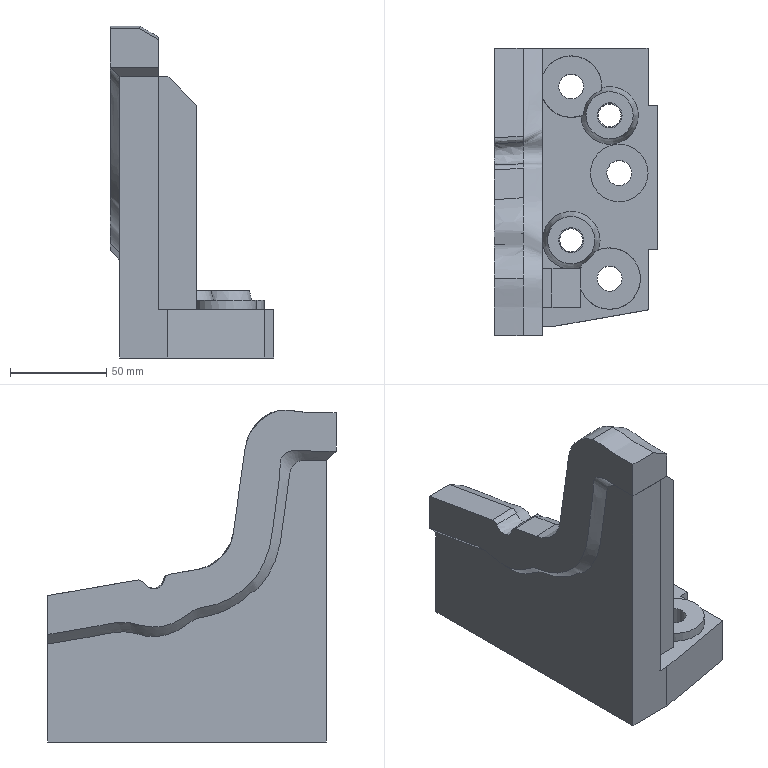Part | NX | features solid 2 | 1 solid | 53 faces | box 85 x 150.07 x 172.946 mm | volume 592103 mm3 | plane 25 | spline 14 | cylinder 12 | cone 2 | commonest cylinder face diameters 13 x5 32 x4 12 x2 30 x1